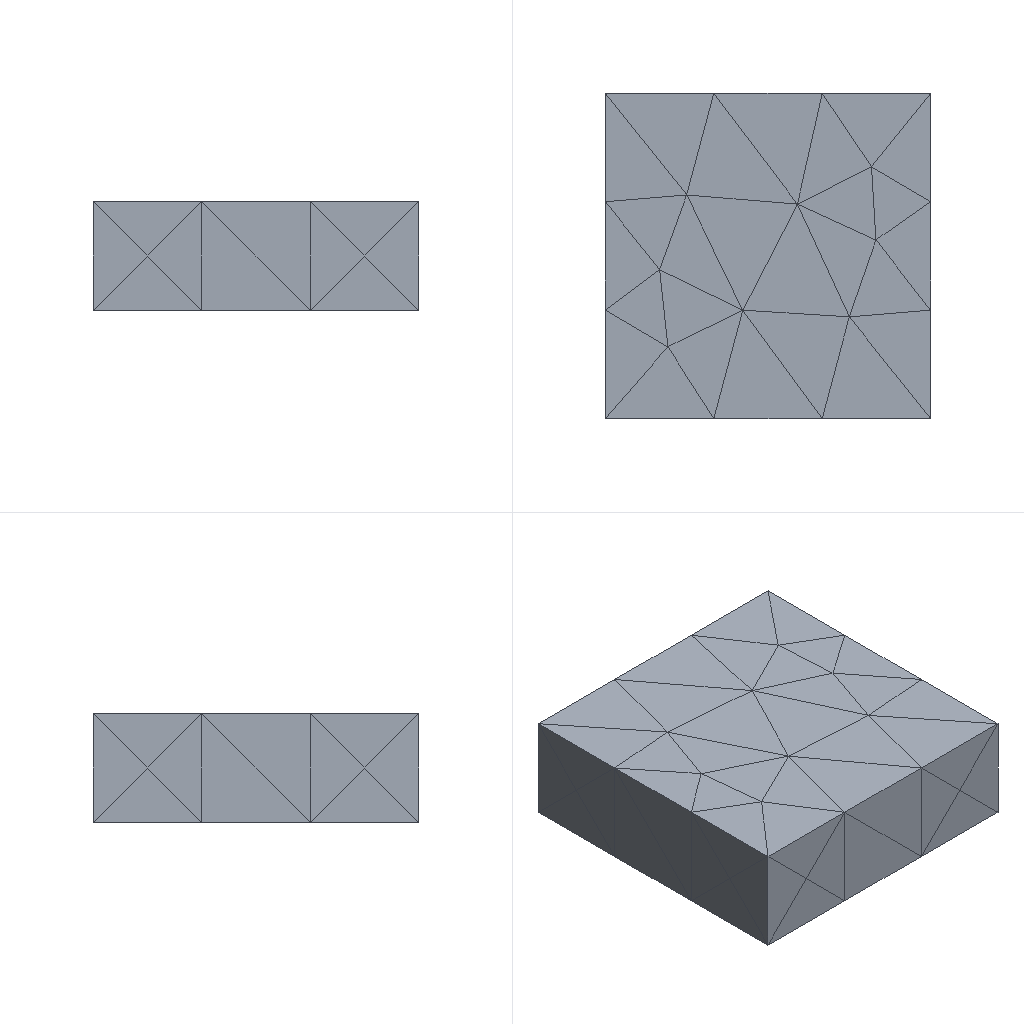Simulation study | ansys mapdl
Set-up summary:
category,name,step,type,value,unit,region
solver,ansys_mapdl
units,mm-N-s-tonne (MPa),,inferred,E=210000 density=
analysis,model,,static
mesh,nodes,,,244
mesh,elements,,,104
element_type,SOLID187,,,104
material,mat 1,,E,210000
material,mat 1,,nu,0.3
load,,model,body load temp,,,all
load,,model,force,"1000 [dir=(0, 0, -1) n=94]",,node list
bc,,model,fixed,"[dofs=UX,UY,UZ n=330]",,node list
Ansys APDL input file, long lists of numbers shortened:
/COM,ANSYS RELEASE 2026 R1           BUILD 26.1      UP20260202       09:04:29
/PREP7
/NOPR
/TITLE,2
ANTYPE, 0
*IF,_CDRDOFF,EQ,1,THEN     !if solid model was read in
_CDRDOFF=             !reset flag, numoffs already performed
*ELSE              !offset database for the following FE model
NUMOFF,NODE,      244
NUMOFF,ELEM,      104
NUMOFF,MAT ,        1
NUMOFF,TYPE,        1
*ENDIF
*SET,_RETURN ,  0.
*SET,_STATUS ,  0.
*SET,_UIQR   ,  94.
*SET,__FLOATPARAMETER__,  244.
DOF,DELETE
ETBLOCK,        1,        1
(2i9,19a9)
        1      187        0        0        0        0        0        0        0        0        0        0        0        0        0        0        0        0        0        0        0
       -1
NBLOCK,6,SOLID,       244,       244
(3i9,6e21.13e3)
        1        0        0 0.0000000000000E+000 3.0000000000000E+001 8.3000000000000E+001
! (243 more lines like these left out)
N,UNBL,LOC,       -1,
EBLOCK,19,SOLID,       104,       104
(19i10)
         1         1         1         1         0         0         0         0        10         0         1       168       141       123        62       184       185       186       162
! (207 more lines like these left out)
        -1
MPTEMP,UNBL, 1, 1,  0.    ,
MPDATA,UNBL, 1,EX  ,       1, 1,  210000.000    ,
MPTEMP,UNBL, 1, 1,  0.    ,
MPDATA,UNBL, 1,NUXY,       1, 1, 0.3    ,
MPTEMP,UNBL, 1, 1,  0.    ,
MPDATA,UNBL, 1,PRXY,       1, 1, 0.3    ,
EXTOPT,ATTR,      0,      0,      0
EXTOPT,ESIZE,  0,  0.
EXTOPT,ACLEAR,      0
TREF,  0.
IRLF,  0
BFUNIF,TEMP,_TINY
ACEL,  0.    ,  0.    ,  0.
OMEGA,  0.    ,  0.    ,  0.
DOMEGA,  0.    ,  0.    ,  0.
CGLOC,  0.    ,  0.    ,  0.
CGOMEGA,  0.    ,  0.    ,  0.
DCGOMG,  0.    ,  0.    ,  0.
KUSE,     0
TIME,  0.
ALPHAD,  0.
BETAD,  0.
DMPRAT,  0.
DMPSTR,  0.
CRPLIM, 0.1    ,   0
CRPLIM,  0.    ,   1
NCNV,     0, 1.000000000E+12,     0,  0.    ,  0.
NEQIT,     0
ERESX,DEFA
DBLOCK,       330
(i9,a6,2(pg16.9))
        1  UX    0.00000000      0.00000000
! (329 more lines like these left out)
       -1
FBLOCK,        94
(i9,a6,2(pg16.9))
       62  FZ   -10.6382979      0.00000000
! (93 more lines like these left out)
       -1
/GO
FINISH
Results summary:
result,analysis_type_db,,,static,unstated
result,n_sets,,,1,unstated
result,load_steps[0].set,load_step=1,,1,unstated
result,load_steps[0].substep,load_step=1,,1,unstated
result,load_steps[0].time,load_step=1,,1,unstated
result,load_steps[0].freq,load_step=1,,1,unstated
result,load_steps[0].max_usum,load_step=1,,0.0001645,unstated
result,load_steps[0].max_seqv,load_step=1,,4.441,unstated
result,load_steps[0].reaction_sum.FX,load_step=1,,4.34941e-12,unstated
result,load_steps[0].reaction_sum.FY,load_step=1,,1.14397e-12,unstated
result,load_steps[0].reaction_sum.FZ,load_step=1,,1000,unstated
result,load_steps[0].reaction_sum.MX,load_step=1,,0,unstated
result,load_steps[0].reaction_sum.MY,load_step=1,,0,unstated
result,load_steps[0].reaction_sum.MZ,load_step=1,,0,unstated
result,convergence,,,results present for all listed sets,unstated